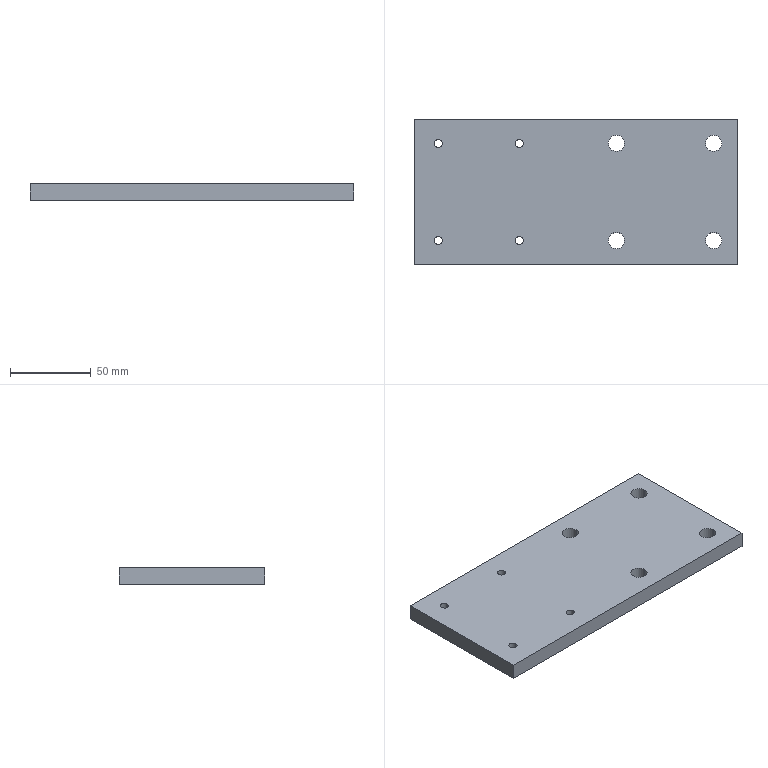Part | SolidWorks | features HoleWzd 2, ICE 2, Extrusion 1 | 1 solid | 22 faces | box 200 x 90 x 10 mm | volume 176073 mm3 | cylinder 16 | plane 6 | commonest cylinder face diameters 5 x8 10 x8
STEP:
#1=CARTESIAN_POINT('',(90.,30.,0.));
#2=VERTEX_POINT('',#1);
#3=CARTESIAN_POINT('',(80.,30.,0.));
#4=VERTEX_POINT('',#3);
#5=CARTESIAN_POINT('',(85.,30.,0.));
#6=DIRECTION('',(0.,0.,-1.));
#7=DIRECTION('',(-1.,0.,0.));
#8=AXIS2_PLACEMENT_3D('',#5,#6,#7);
#9=CIRCLE('',#8,5.);
#10=EDGE_CURVE('',#2,#4,#9,.T.);
#11=ORIENTED_EDGE('',*,*,#10,.T.);
#12=CARTESIAN_POINT('',(80.,30.,10.));
#13=VERTEX_POINT('',#12);
#14=CARTESIAN_POINT('',(80.,30.,10.));
#15=DIRECTION('',(0.,0.,1.));
#16=VECTOR('',#15,1000.);
#17=LINE('',#14,#16);
#18=EDGE_CURVE('',#4,#13,#17,.T.);
#19=ORIENTED_EDGE('',*,*,#18,.T.);
#20=CARTESIAN_POINT('',(90.,30.,10.));
#21=VERTEX_POINT('',#20);
#22=CARTESIAN_POINT('',(85.,30.,10.));
#23=DIRECTION('',(0.,0.,1.));
#24=DIRECTION('',(1.,0.,0.));
#25=AXIS2_PLACEMENT_3D('',#22,#23,#24);
#26=CIRCLE('',#25,5.);
#27=EDGE_CURVE('',#13,#21,#26,.T.);
#28=ORIENTED_EDGE('',*,*,#27,.T.);
#29=CARTESIAN_POINT('',(90.,30.,10.));
#30=DIRECTION('',(0.,0.,1.));
#31=VECTOR('',#30,1000.);
#32=LINE('',#29,#31);
#33=EDGE_CURVE('',#2,#21,#32,.T.);
#34=ORIENTED_EDGE('',*,*,#33,.F.);
#35=EDGE_LOOP('',(#11,#19,#28,#34));
#36=FACE_OUTER_BOUND('',#35,.T.);
#37=CARTESIAN_POINT('',(85.,30.,10.));
#38=DIRECTION('',(0.,0.,1.));
#39=DIRECTION('',(1.,0.,0.));
#40=AXIS2_PLACEMENT_3D('',#37,#38,#39);
#41=CYLINDRICAL_SURFACE('',#40,5.);
#42=ADVANCED_FACE('',(#36),#41,.F.);
#43=CARTESIAN_POINT('',(30.,-30.,0.));
#44=VERTEX_POINT('',#43);
#45=CARTESIAN_POINT('',(20.,-30.,0.));
#46=VERTEX_POINT('',#45);
#47=CARTESIAN_POINT('',(25.,-30.,0.));
#48=DIRECTION('',(0.,0.,-1.));
#49=DIRECTION('',(-1.,0.,0.));
#50=AXIS2_PLACEMENT_3D('',#47,#48,#49);
#51=CIRCLE('',#50,5.);
#52=EDGE_CURVE('',#44,#46,#51,.T.);
#53=ORIENTED_EDGE('',*,*,#52,.T.);
#54=CARTESIAN_POINT('',(20.,-30.,10.));
#55=VERTEX_POINT('',#54);
#56=CARTESIAN_POINT('',(20.,-30.,10.));
#57=DIRECTION('',(0.,0.,1.));
#58=VECTOR('',#57,1000.);
#59=LINE('',#56,#58);
#60=EDGE_CURVE('',#46,#55,#59,.T.);
#61=ORIENTED_EDGE('',*,*,#60,.T.);
#62=CARTESIAN_POINT('',(30.,-30.,10.));
#63=VERTEX_POINT('',#62);
#64=CARTESIAN_POINT('',(25.,-30.,10.));
#65=DIRECTION('',(0.,0.,1.));
#66=DIRECTION('',(1.,0.,0.));
#67=AXIS2_PLACEMENT_3D('',#64,#65,#66);
#68=CIRCLE('',#67,5.);
#69=EDGE_CURVE('',#55,#63,#68,.T.);
#70=ORIENTED_EDGE('',*,*,#69,.T.);
#71=CARTESIAN_POINT('',(30.,-30.,10.));
#72=DIRECTION('',(0.,0.,1.));
#73=VECTOR('',#72,1000.);
#74=LINE('',#71,#73);
#75=EDGE_CURVE('',#44,#63,#74,.T.);
#76=ORIENTED_EDGE('',*,*,#75,.F.);
#77=EDGE_LOOP('',(#53,#61,#70,#76));
#78=FACE_OUTER_BOUND('',#77,.T.);
#79=CARTESIAN_POINT('',(25.,-30.,10.));
#80=DIRECTION('',(0.,0.,1.));
#81=DIRECTION('',(1.,0.,0.));
#82=AXIS2_PLACEMENT_3D('',#79,#80,#81);
#83=CYLINDRICAL_SURFACE('',#82,5.);
#84=ADVANCED_FACE('',(#78),#83,.F.);
#85=CARTESIAN_POINT('',(30.,30.,0.));
#86=VERTEX_POINT('',#85);
#87=CARTESIAN_POINT('',(20.,30.,0.));
#88=VERTEX_POINT('',#87);
#89=CARTESIAN_POINT('',(25.,30.,0.));
#90=DIRECTION('',(0.,0.,-1.));
#91=DIRECTION('',(-1.,0.,0.));
#92=AXIS2_PLACEMENT_3D('',#89,#90,#91);
#93=CIRCLE('',#92,5.);
#94=EDGE_CURVE('',#86,#88,#93,.T.);
#95=ORIENTED_EDGE('',*,*,#94,.T.);
#96=CARTESIAN_POINT('',(20.,30.,10.));
#97=VERTEX_POINT('',#96);
#98=CARTESIAN_POINT('',(20.,30.,10.));
#99=DIRECTION('',(0.,0.,1.));
#100=VECTOR('',#99,1000.);
#101=LINE('',#98,#100);
#102=EDGE_CURVE('',#88,#97,#101,.T.);
#103=ORIENTED_EDGE('',*,*,#102,.T.);
#104=CARTESIAN_POINT('',(30.,30.,10.));
#105=VERTEX_POINT('',#104);
#106=CARTESIAN_POINT('',(25.,30.,10.));
#107=DIRECTION('',(0.,0.,1.));
#108=DIRECTION('',(1.,0.,0.));
#109=AXIS2_PLACEMENT_3D('',#106,#107,#108);
#110=CIRCLE('',#109,5.);
#111=EDGE_CURVE('',#97,#105,#110,.T.);
#112=ORIENTED_EDGE('',*,*,#111,.T.);
#113=CARTESIAN_POINT('',(30.,30.,10.));
#114=DIRECTION('',(0.,0.,1.));
#115=VECTOR('',#114,1000.);
#116=LINE('',#113,#115);
#117=EDGE_CURVE('',#86,#105,#116,.T.);
#118=ORIENTED_EDGE('',*,*,#117,.F.);
#119=EDGE_LOOP('',(#95,#103,#112,#118));
#120=FACE_OUTER_BOUND('',#119,.T.);
#121=CARTESIAN_POINT('',(25.,30.,10.));
#122=DIRECTION('',(0.,0.,1.));
#123=DIRECTION('',(1.,0.,0.));
#124=AXIS2_PLACEMENT_3D('',#121,#122,#123);
#125=CYLINDRICAL_SURFACE('',#124,5.);
#126=ADVANCED_FACE('',(#120),#125,.F.);
#127=CARTESIAN_POINT('',(90.,-30.,0.));
#128=VERTEX_POINT('',#127);
#129=CARTESIAN_POINT('',(80.,-30.,0.));
#130=VERTEX_POINT('',#129);
#131=CARTESIAN_POINT('',(85.,-30.,0.));
#132=DIRECTION('',(0.,0.,-1.));
#133=DIRECTION('',(-1.,0.,0.));
#134=AXIS2_PLACEMENT_3D('',#131,#132,#133);
#135=CIRCLE('',#134,5.);
#136=EDGE_CURVE('',#128,#130,#135,.T.);
#137=ORIENTED_EDGE('',*,*,#136,.T.);
#138=CARTESIAN_POINT('',(80.,-30.,10.));
#139=VERTEX_POINT('',#138);
#140=CARTESIAN_POINT('',(80.,-30.,10.));
#141=DIRECTION('',(0.,0.,1.));
#142=VECTOR('',#141,1000.);
#143=LINE('',#140,#142);
#144=EDGE_CURVE('',#130,#139,#143,.T.);
#145=ORIENTED_EDGE('',*,*,#144,.T.);
#146=CARTESIAN_POINT('',(90.,-30.,10.));
#147=VERTEX_POINT('',#146);
#148=CARTESIAN_POINT('',(85.,-30.,10.));
#149=DIRECTION('',(0.,0.,1.));
#150=DIRECTION('',(1.,0.,0.));
#151=AXIS2_PLACEMENT_3D('',#148,#149,#150);
#152=CIRCLE('',#151,5.);
#153=EDGE_CURVE('',#139,#147,#152,.T.);
#154=ORIENTED_EDGE('',*,*,#153,.T.);
#155=CARTESIAN_POINT('',(90.,-30.,10.));
#156=DIRECTION('',(0.,0.,1.));
#157=VECTOR('',#156,1000.);
#158=LINE('',#155,#157);
#159=EDGE_CURVE('',#128,#147,#158,.T.);
#160=ORIENTED_EDGE('',*,*,#159,.F.);
#161=EDGE_LOOP('',(#137,#145,#154,#160));
#162=FACE_OUTER_BOUND('',#161,.T.);
#163=CARTESIAN_POINT('',(85.,-30.,10.));
#164=DIRECTION('',(0.,0.,1.));
#165=DIRECTION('',(1.,0.,0.));
#166=AXIS2_PLACEMENT_3D('',#163,#164,#165);
#167=CYLINDRICAL_SURFACE('',#166,5.);
#168=ADVANCED_FACE('',(#162),#167,.F.);
#169=CARTESIAN_POINT('',(-32.5,-30.,10.));
#170=VERTEX_POINT('',#169);
#171=CARTESIAN_POINT('',(-37.5,-30.,10.));
#172=VERTEX_POINT('',#171);
#173=CARTESIAN_POINT('',(-35.,-30.,10.));
#174=DIRECTION('',(0.,0.,-1.));
#175=DIRECTION('',(-1.,0.,0.));
#176=AXIS2_PLACEMENT_3D('',#173,#174,#175);
#177=CIRCLE('',#176,2.5);
#178=EDGE_CURVE('',#170,#172,#177,.T.);
#179=ORIENTED_EDGE('',*,*,#178,.F.);
#180=CARTESIAN_POINT('',(-32.5,-30.,0.));
#181=VERTEX_POINT('',#180);
#182=CARTESIAN_POINT('',(-32.5,-30.,0.));
#183=DIRECTION('',(0.,0.,-1.));
#184=VECTOR('',#183,1000.);
#185=LINE('',#182,#184);
#186=EDGE_CURVE('',#170,#181,#185,.T.);
#187=ORIENTED_EDGE('',*,*,#186,.T.);
#188=CARTESIAN_POINT('',(-37.5,-30.,0.));
#189=VERTEX_POINT('',#188);
#190=CARTESIAN_POINT('',(-35.,-30.,0.));
#191=DIRECTION('',(0.,0.,-1.));
#192=DIRECTION('',(-1.,0.,0.));
#193=AXIS2_PLACEMENT_3D('',#190,#191,#192);
#194=CIRCLE('',#193,2.5);
#195=EDGE_CURVE('',#181,#189,#194,.T.);
#196=ORIENTED_EDGE('',*,*,#195,.T.);
#197=CARTESIAN_POINT('',(-37.5,-30.,0.));
#198=DIRECTION('',(0.,0.,-1.));
#199=VECTOR('',#198,1000.);
#200=LINE('',#197,#199);
#201=EDGE_CURVE('',#172,#189,#200,.T.);
#202=ORIENTED_EDGE('',*,*,#201,.F.);
#203=EDGE_LOOP('',(#179,#187,#196,#202));
#204=FACE_OUTER_BOUND('',#203,.T.);
#205=CARTESIAN_POINT('',(-35.,-30.,0.));
#206=DIRECTION('',(0.,0.,-1.));
#207=DIRECTION('',(-1.,0.,0.));
#208=AXIS2_PLACEMENT_3D('',#205,#206,#207);
#209=CYLINDRICAL_SURFACE('',#208,2.5);
#210=ADVANCED_FACE('',(#204),#209,.F.);
#211=CARTESIAN_POINT('',(-82.5,-30.,10.));
#212=VERTEX_POINT('',#211);
#213=CARTESIAN_POINT('',(-87.5,-30.,10.));
#214=VERTEX_POINT('',#213);
#215=CARTESIAN_POINT('',(-85.,-30.,10.));
#216=DIRECTION('',(0.,0.,-1.));
#217=DIRECTION('',(-1.,0.,0.));
#218=AXIS2_PLACEMENT_3D('',#215,#216,#217);
#219=CIRCLE('',#218,2.5);
#220=EDGE_CURVE('',#212,#214,#219,.T.);
#221=ORIENTED_EDGE('',*,*,#220,.F.);
#222=CARTESIAN_POINT('',(-82.5,-30.,0.));
#223=VERTEX_POINT('',#222);
#224=CARTESIAN_POINT('',(-82.5,-30.,0.));
#225=DIRECTION('',(0.,0.,-1.));
#226=VECTOR('',#225,1000.);
#227=LINE('',#224,#226);
#228=EDGE_CURVE('',#212,#223,#227,.T.);
#229=ORIENTED_EDGE('',*,*,#228,.T.);
#230=CARTESIAN_POINT('',(-87.5,-30.,0.));
#231=VERTEX_POINT('',#230);
#232=CARTESIAN_POINT('',(-85.,-30.,0.));
#233=DIRECTION('',(0.,0.,-1.));
#234=DIRECTION('',(-1.,0.,0.));
#235=AXIS2_PLACEMENT_3D('',#232,#233,#234);
#236=CIRCLE('',#235,2.5);
#237=EDGE_CURVE('',#223,#231,#236,.T.);
#238=ORIENTED_EDGE('',*,*,#237,.T.);
#239=CARTESIAN_POINT('',(-87.5,-30.,0.));
#240=DIRECTION('',(0.,0.,-1.));
#241=VECTOR('',#240,1000.);
#242=LINE('',#239,#241);
#243=EDGE_CURVE('',#214,#231,#242,.T.);
#244=ORIENTED_EDGE('',*,*,#243,.F.);
#245=EDGE_LOOP('',(#221,#229,#238,#244));
#246=FACE_OUTER_BOUND('',#245,.T.);
#247=CARTESIAN_POINT('',(-85.,-30.,0.));
#248=DIRECTION('',(0.,0.,-1.));
#249=DIRECTION('',(-1.,0.,0.));
#250=AXIS2_PLACEMENT_3D('',#247,#248,#249);
#251=CYLINDRICAL_SURFACE('',#250,2.5);
#252=ADVANCED_FACE('',(#246),#251,.F.);
#253=CARTESIAN_POINT('',(-32.5,30.,10.));
#254=VERTEX_POINT('',#253);
#255=CARTESIAN_POINT('',(-37.5,30.,10.));
#256=VERTEX_POINT('',#255);
#257=CARTESIAN_POINT('',(-35.,30.,10.));
#258=DIRECTION('',(0.,0.,-1.));
#259=DIRECTION('',(-1.,0.,0.));
#260=AXIS2_PLACEMENT_3D('',#257,#258,#259);
#261=CIRCLE('',#260,2.5);
#262=EDGE_CURVE('',#254,#256,#261,.T.);
#263=ORIENTED_EDGE('',*,*,#262,.F.);
#264=CARTESIAN_POINT('',(-32.5,30.,0.));
#265=VERTEX_POINT('',#264);
#266=CARTESIAN_POINT('',(-32.5,30.,0.));
#267=DIRECTION('',(0.,0.,-1.));
#268=VECTOR('',#267,1000.);
#269=LINE('',#266,#268);
#270=EDGE_CURVE('',#254,#265,#269,.T.);
#271=ORIENTED_EDGE('',*,*,#270,.T.);
#272=CARTESIAN_POINT('',(-37.5,30.,0.));
#273=VERTEX_POINT('',#272);
#274=CARTESIAN_POINT('',(-35.,30.,0.));
#275=DIRECTION('',(0.,0.,-1.));
#276=DIRECTION('',(-1.,0.,0.));
#277=AXIS2_PLACEMENT_3D('',#274,#275,#276);
#278=CIRCLE('',#277,2.5);
#279=EDGE_CURVE('',#265,#273,#278,.T.);
#280=ORIENTED_EDGE('',*,*,#279,.T.);
#281=CARTESIAN_POINT('',(-37.5,30.,0.));
#282=DIRECTION('',(0.,0.,-1.));
#283=VECTOR('',#282,1000.);
#284=LINE('',#281,#283);
#285=EDGE_CURVE('',#256,#273,#284,.T.);
#286=ORIENTED_EDGE('',*,*,#285,.F.);
#287=EDGE_LOOP('',(#263,#271,#280,#286));
#288=FACE_OUTER_BOUND('',#287,.T.);
#289=CARTESIAN_POINT('',(-35.,30.,0.));
#290=DIRECTION('',(0.,0.,-1.));
#291=DIRECTION('',(-1.,0.,0.));
#292=AXIS2_PLACEMENT_3D('',#289,#290,#291);
#293=CYLINDRICAL_SURFACE('',#292,2.5);
#294=ADVANCED_FACE('',(#288),#293,.F.);
#295=CARTESIAN_POINT('',(-82.5,30.,10.));
#296=VERTEX_POINT('',#295);
#297=CARTESIAN_POINT('',(-87.5,30.,10.));
#298=VERTEX_POINT('',#297);
#299=CARTESIAN_POINT('',(-85.,30.,10.));
#300=DIRECTION('',(0.,0.,-1.));
#301=DIRECTION('',(-1.,0.,0.));
#302=AXIS2_PLACEMENT_3D('',#299,#300,#301);
#303=CIRCLE('',#302,2.5);
#304=EDGE_CURVE('',#296,#298,#303,.T.);
#305=ORIENTED_EDGE('',*,*,#304,.F.);
#306=CARTESIAN_POINT('',(-82.5,30.,0.));
#307=VERTEX_POINT('',#306);
#308=CARTESIAN_POINT('',(-82.5,30.,0.));
#309=DIRECTION('',(0.,0.,-1.));
#310=VECTOR('',#309,1000.);
#311=LINE('',#308,#310);
#312=EDGE_CURVE('',#296,#307,#311,.T.);
#313=ORIENTED_EDGE('',*,*,#312,.T.);
#314=CARTESIAN_POINT('',(-87.5,30.,0.));
#315=VERTEX_POINT('',#314);
#316=CARTESIAN_POINT('',(-85.,30.,0.));
#317=DIRECTION('',(0.,0.,-1.));
#318=DIRECTION('',(-1.,0.,0.));
#319=AXIS2_PLACEMENT_3D('',#316,#317,#318);
#320=CIRCLE('',#319,2.5);
#321=EDGE_CURVE('',#307,#315,#320,.T.);
#322=ORIENTED_EDGE('',*,*,#321,.T.);
#323=CARTESIAN_POINT('',(-87.5,30.,0.));
#324=DIRECTION('',(0.,0.,-1.));
#325=VECTOR('',#324,1000.);
#326=LINE('',#323,#325);
#327=EDGE_CURVE('',#298,#315,#326,.T.);
#328=ORIENTED_EDGE('',*,*,#327,.F.);
#329=EDGE_LOOP('',(#305,#313,#322,#328));
#330=FACE_OUTER_BOUND('',#329,.T.);
#331=CARTESIAN_POINT('',(-85.,30.,0.));
#332=DIRECTION('',(0.,0.,-1.));
#333=DIRECTION('',(-1.,0.,0.));
#334=AXIS2_PLACEMENT_3D('',#331,#332,#333);
#335=CYLINDRICAL_SURFACE('',#334,2.5);
#336=ADVANCED_FACE('',(#330),#335,.F.);
#337=CARTESIAN_POINT('',(100.,-45.,0.));
#338=VERTEX_POINT('',#337);
#339=CARTESIAN_POINT('',(100.,45.,0.));
#340=VERTEX_POINT('',#339);
#341=CARTESIAN_POINT('',(100.,-45.,0.));
#342=DIRECTION('',(0.,1.,0.));
#343=VECTOR('',#342,1000.);
#344=LINE('',#341,#343);
#345=EDGE_CURVE('',#338,#340,#344,.T.);
#346=ORIENTED_EDGE('',*,*,#345,.T.);
#347=CARTESIAN_POINT('',(100.,45.,10.));
#348=VERTEX_POINT('',#347);
#349=CARTESIAN_POINT('',(100.,45.,10.));
#350=DIRECTION('',(0.,0.,-1.));
#351=VECTOR('',#350,1000.);
#352=LINE('',#349,#351);
#353=EDGE_CURVE('',#348,#340,#352,.T.);
#354=ORIENTED_EDGE('',*,*,#353,.F.);
#355=CARTESIAN_POINT('',(100.,-45.,10.));
#356=VERTEX_POINT('',#355);
#357=CARTESIAN_POINT('',(100.,-45.,10.));
#358=DIRECTION('',(0.,1.,0.));
#359=VECTOR('',#358,1000.);
#360=LINE('',#357,#359);
#361=EDGE_CURVE('',#356,#348,#360,.T.);
#362=ORIENTED_EDGE('',*,*,#361,.F.);
#363=CARTESIAN_POINT('',(100.,-45.,10.));
#364=DIRECTION('',(0.,0.,-1.));
#365=VECTOR('',#364,1000.);
#366=LINE('',#363,#365);
#367=EDGE_CURVE('',#356,#338,#366,.T.);
#368=ORIENTED_EDGE('',*,*,#367,.T.);
#369=EDGE_LOOP('',(#346,#354,#362,#368));
#370=FACE_OUTER_BOUND('',#369,.T.);
#371=CARTESIAN_POINT('',(100.,-45.,10.));
#372=DIRECTION('',(-1.,0.,0.));
#373=DIRECTION('',(0.,0.,1.));
#374=AXIS2_PLACEMENT_3D('',#371,#372,#373);
#375=PLANE('',#374);
#376=ADVANCED_FACE('',(#370),#375,.F.);
#377=CARTESIAN_POINT('',(-100.,45.,0.));
#378=VERTEX_POINT('',#377);
#379=CARTESIAN_POINT('',(-100.,45.,0.));
#380=DIRECTION('',(-1.,0.,0.));
#381=VECTOR('',#380,1000.);
#382=LINE('',#379,#381);
#383=EDGE_CURVE('',#340,#378,#382,.T.);
#384=ORIENTED_EDGE('',*,*,#383,.T.);
#385=CARTESIAN_POINT('',(-100.,45.,10.));
#386=VERTEX_POINT('',#385);
#387=CARTESIAN_POINT('',(-100.,45.,10.));
#388=DIRECTION('',(0.,0.,-1.));
#389=VECTOR('',#388,1000.);
#390=LINE('',#387,#389);
#391=EDGE_CURVE('',#386,#378,#390,.T.);
#392=ORIENTED_EDGE('',*,*,#391,.F.);
#393=CARTESIAN_POINT('',(-100.,45.,10.));
#394=DIRECTION('',(-1.,0.,0.));
#395=VECTOR('',#394,1000.);
#396=LINE('',#393,#395);
#397=EDGE_CURVE('',#348,#386,#396,.T.);
#398=ORIENTED_EDGE('',*,*,#397,.F.);
#399=ORIENTED_EDGE('',*,*,#353,.T.);
#400=EDGE_LOOP('',(#384,#392,#398,#399));
#401=FACE_OUTER_BOUND('',#400,.T.);
#402=CARTESIAN_POINT('',(-100.,45.,10.));
#403=DIRECTION('',(0.,-1.,0.));
#404=DIRECTION('',(0.,0.,-1.));
#405=AXIS2_PLACEMENT_3D('',#402,#403,#404);
#406=PLANE('',#405);
#407=ADVANCED_FACE('',(#401),#406,.F.);
#408=CARTESIAN_POINT('',(-100.,-45.,0.));
#409=VERTEX_POINT('',#408);
#410=CARTESIAN_POINT('',(-100.,-45.,0.));
#411=DIRECTION('',(0.,-1.,0.));
#412=VECTOR('',#411,1000.);
#413=LINE('',#410,#412);
#414=EDGE_CURVE('',#378,#409,#413,.T.);
#415=ORIENTED_EDGE('',*,*,#414,.T.);
#416=CARTESIAN_POINT('',(-100.,-45.,10.));
#417=VERTEX_POINT('',#416);
#418=CARTESIAN_POINT('',(-100.,-45.,10.));
#419=DIRECTION('',(0.,0.,-1.));
#420=VECTOR('',#419,1000.);
#421=LINE('',#418,#420);
#422=EDGE_CURVE('',#417,#409,#421,.T.);
#423=ORIENTED_EDGE('',*,*,#422,.F.);
#424=CARTESIAN_POINT('',(-100.,-45.,10.));
#425=DIRECTION('',(0.,-1.,0.));
#426=VECTOR('',#425,1000.);
#427=LINE('',#424,#426);
#428=EDGE_CURVE('',#386,#417,#427,.T.);
#429=ORIENTED_EDGE('',*,*,#428,.F.);
#430=ORIENTED_EDGE('',*,*,#391,.T.);
#431=EDGE_LOOP('',(#415,#423,#429,#430));
#432=FACE_OUTER_BOUND('',#431,.T.);
#433=CARTESIAN_POINT('',(-100.,-45.,10.));
#434=DIRECTION('',(1.,0.,0.));
#435=DIRECTION('',(0.,0.,-1.));
#436=AXIS2_PLACEMENT_3D('',#433,#434,#435);
#437=PLANE('',#436);
#438=ADVANCED_FACE('',(#432),#437,.F.);
#439=CARTESIAN_POINT('',(-100.,-45.,0.));
#440=DIRECTION('',(1.,0.,0.));
#441=VECTOR('',#440,1000.);
#442=LINE('',#439,#441);
#443=EDGE_CURVE('',#409,#338,#442,.T.);
#444=ORIENTED_EDGE('',*,*,#443,.T.);
#445=ORIENTED_EDGE('',*,*,#367,.F.);
#446=CARTESIAN_POINT('',(-100.,-45.,10.));
#447=DIRECTION('',(1.,0.,0.));
#448=VECTOR('',#447,1000.);
#449=LINE('',#446,#448);
#450=EDGE_CURVE('',#417,#356,#449,.T.);
#451=ORIENTED_EDGE('',*,*,#450,.F.);
#452=ORIENTED_EDGE('',*,*,#422,.T.);
#453=EDGE_LOOP('',(#444,#445,#451,#452));
#454=FACE_OUTER_BOUND('',#453,.T.);
#455=CARTESIAN_POINT('',(-100.,-45.,10.));
#456=DIRECTION('',(0.,1.,0.));
#457=DIRECTION('',(0.,0.,1.));
#458=AXIS2_PLACEMENT_3D('',#455,#456,#457);
#459=PLANE('',#458);
#460=ADVANCED_FACE('',(#454),#459,.F.);
#461=CARTESIAN_POINT('',(85.,30.,10.));
#462=DIRECTION('',(0.,0.,1.));
#463=DIRECTION('',(1.,0.,0.));
#464=AXIS2_PLACEMENT_3D('',#461,#462,#463);
#465=CIRCLE('',#464,5.);
#466=EDGE_CURVE('',#21,#13,#465,.T.);
#467=ORIENTED_EDGE('',*,*,#466,.F.);
#468=ORIENTED_EDGE('',*,*,#27,.F.);
#469=EDGE_LOOP('',(#467,#468));
#470=FACE_BOUND('',#469,.T.);
#471=CARTESIAN_POINT('',(25.,-30.,10.));
#472=DIRECTION('',(0.,0.,1.));
#473=DIRECTION('',(1.,0.,0.));
#474=AXIS2_PLACEMENT_3D('',#471,#472,#473);
#475=CIRCLE('',#474,5.);
#476=EDGE_CURVE('',#63,#55,#475,.T.);
#477=ORIENTED_EDGE('',*,*,#476,.F.);
#478=ORIENTED_EDGE('',*,*,#69,.F.);
#479=EDGE_LOOP('',(#477,#478));
#480=FACE_BOUND('',#479,.T.);
#481=CARTESIAN_POINT('',(25.,30.,10.));
#482=DIRECTION('',(0.,0.,1.));
#483=DIRECTION('',(1.,0.,0.));
#484=AXIS2_PLACEMENT_3D('',#481,#482,#483);
#485=CIRCLE('',#484,5.);
#486=EDGE_CURVE('',#105,#97,#485,.T.);
#487=ORIENTED_EDGE('',*,*,#486,.F.);
#488=ORIENTED_EDGE('',*,*,#111,.F.);
#489=EDGE_LOOP('',(#487,#488));
#490=FACE_BOUND('',#489,.T.);
#491=CARTESIAN_POINT('',(85.,-30.,10.));
#492=DIRECTION('',(0.,0.,1.));
#493=DIRECTION('',(1.,0.,0.));
#494=AXIS2_PLACEMENT_3D('',#491,#492,#493);
#495=CIRCLE('',#494,5.);
#496=EDGE_CURVE('',#147,#139,#495,.T.);
#497=ORIENTED_EDGE('',*,*,#496,.F.);
#498=ORIENTED_EDGE('',*,*,#153,.F.);
#499=EDGE_LOOP('',(#497,#498));
#500=FACE_BOUND('',#499,.T.);
#501=CARTESIAN_POINT('',(-35.,-30.,10.));
#502=DIRECTION('',(0.,0.,-1.));
#503=DIRECTION('',(-1.,0.,0.));
#504=AXIS2_PLACEMENT_3D('',#501,#502,#503);
#505=CIRCLE('',#504,2.5);
#506=EDGE_CURVE('',#172,#170,#505,.T.);
#507=ORIENTED_EDGE('',*,*,#506,.T.);
#508=ORIENTED_EDGE('',*,*,#178,.T.);
#509=EDGE_LOOP('',(#507,#508));
#510=FACE_BOUND('',#509,.T.);
#511=CARTESIAN_POINT('',(-85.,-30.,10.));
#512=DIRECTION('',(0.,0.,-1.));
#513=DIRECTION('',(-1.,0.,0.));
#514=AXIS2_PLACEMENT_3D('',#511,#512,#513);
#515=CIRCLE('',#514,2.5);
#516=EDGE_CURVE('',#214,#212,#515,.T.);
#517=ORIENTED_EDGE('',*,*,#516,.T.);
#518=ORIENTED_EDGE('',*,*,#220,.T.);
#519=EDGE_LOOP('',(#517,#518));
#520=FACE_BOUND('',#519,.T.);
#521=CARTESIAN_POINT('',(-35.,30.,10.));
#522=DIRECTION('',(0.,0.,-1.));
#523=DIRECTION('',(-1.,0.,0.));
#524=AXIS2_PLACEMENT_3D('',#521,#522,#523);
#525=CIRCLE('',#524,2.5);
#526=EDGE_CURVE('',#256,#254,#525,.T.);
#527=ORIENTED_EDGE('',*,*,#526,.T.);
#528=ORIENTED_EDGE('',*,*,#262,.T.);
#529=EDGE_LOOP('',(#527,#528));
#530=FACE_BOUND('',#529,.T.);
#531=CARTESIAN_POINT('',(-85.,30.,10.));
#532=DIRECTION('',(0.,0.,-1.));
#533=DIRECTION('',(-1.,0.,0.));
#534=AXIS2_PLACEMENT_3D('',#531,#532,#533);
#535=CIRCLE('',#534,2.5);
#536=EDGE_CURVE('',#298,#296,#535,.T.);
#537=ORIENTED_EDGE('',*,*,#536,.T.);
#538=ORIENTED_EDGE('',*,*,#304,.T.);
#539=EDGE_LOOP('',(#537,#538));
#540=FACE_BOUND('',#539,.T.);
#541=ORIENTED_EDGE('',*,*,#361,.T.);
#542=ORIENTED_EDGE('',*,*,#397,.T.);
#543=ORIENTED_EDGE('',*,*,#428,.T.);
#544=ORIENTED_EDGE('',*,*,#450,.T.);
#545=EDGE_LOOP('',(#541,#542,#543,#544));
#546=FACE_OUTER_BOUND('',#545,.T.);
#547=CARTESIAN_POINT('',(0.,0.,10.));
#548=DIRECTION('',(0.,0.,-1.));
#549=DIRECTION('',(-1.,0.,0.));
#550=AXIS2_PLACEMENT_3D('',#547,#548,#549);
#551=PLANE('',#550);
#552=ADVANCED_FACE('',(#470,#480,#490,#500,#510,#520,#530,#540,#546),#551,.F.);
#553=ORIENTED_EDGE('',*,*,#10,.F.);
#554=CARTESIAN_POINT('',(85.,30.,0.));
#555=DIRECTION('',(0.,0.,-1.));
#556=DIRECTION('',(-1.,0.,0.));
#557=AXIS2_PLACEMENT_3D('',#554,#555,#556);
#558=CIRCLE('',#557,5.);
#559=EDGE_CURVE('',#4,#2,#558,.T.);
#560=ORIENTED_EDGE('',*,*,#559,.F.);
#561=EDGE_LOOP('',(#553,#560));
#562=FACE_BOUND('',#561,.T.);
#563=ORIENTED_EDGE('',*,*,#52,.F.);
#564=CARTESIAN_POINT('',(25.,-30.,0.));
#565=DIRECTION('',(0.,0.,-1.));
#566=DIRECTION('',(-1.,0.,0.));
#567=AXIS2_PLACEMENT_3D('',#564,#565,#566);
#568=CIRCLE('',#567,5.);
#569=EDGE_CURVE('',#46,#44,#568,.T.);
#570=ORIENTED_EDGE('',*,*,#569,.F.);
#571=EDGE_LOOP('',(#563,#570));
#572=FACE_BOUND('',#571,.T.);
#573=ORIENTED_EDGE('',*,*,#94,.F.);
#574=CARTESIAN_POINT('',(25.,30.,0.));
#575=DIRECTION('',(0.,0.,-1.));
#576=DIRECTION('',(-1.,0.,0.));
#577=AXIS2_PLACEMENT_3D('',#574,#575,#576);
#578=CIRCLE('',#577,5.);
#579=EDGE_CURVE('',#88,#86,#578,.T.);
#580=ORIENTED_EDGE('',*,*,#579,.F.);
#581=EDGE_LOOP('',(#573,#580));
#582=FACE_BOUND('',#581,.T.);
#583=ORIENTED_EDGE('',*,*,#136,.F.);
#584=CARTESIAN_POINT('',(85.,-30.,0.));
#585=DIRECTION('',(0.,0.,-1.));
#586=DIRECTION('',(-1.,0.,0.));
#587=AXIS2_PLACEMENT_3D('',#584,#585,#586);
#588=CIRCLE('',#587,5.);
#589=EDGE_CURVE('',#130,#128,#588,.T.);
#590=ORIENTED_EDGE('',*,*,#589,.F.);
#591=EDGE_LOOP('',(#583,#590));
#592=FACE_BOUND('',#591,.T.);
#593=CARTESIAN_POINT('',(-35.,-30.,0.));
#594=DIRECTION('',(0.,0.,-1.));
#595=DIRECTION('',(-1.,0.,0.));
#596=AXIS2_PLACEMENT_3D('',#593,#594,#595);
#597=CIRCLE('',#596,2.5);
#598=EDGE_CURVE('',#189,#181,#597,.T.);
#599=ORIENTED_EDGE('',*,*,#598,.F.);
#600=ORIENTED_EDGE('',*,*,#195,.F.);
#601=EDGE_LOOP('',(#599,#600));
#602=FACE_BOUND('',#601,.T.);
#603=CARTESIAN_POINT('',(-85.,-30.,0.));
#604=DIRECTION('',(0.,0.,-1.));
#605=DIRECTION('',(-1.,0.,0.));
#606=AXIS2_PLACEMENT_3D('',#603,#604,#605);
#607=CIRCLE('',#606,2.5);
#608=EDGE_CURVE('',#231,#223,#607,.T.);
#609=ORIENTED_EDGE('',*,*,#608,.F.);
#610=ORIENTED_EDGE('',*,*,#237,.F.);
#611=EDGE_LOOP('',(#609,#610));
#612=FACE_BOUND('',#611,.T.);
#613=CARTESIAN_POINT('',(-35.,30.,0.));
#614=DIRECTION('',(0.,0.,-1.));
#615=DIRECTION('',(-1.,0.,0.));
#616=AXIS2_PLACEMENT_3D('',#613,#614,#615);
#617=CIRCLE('',#616,2.5);
#618=EDGE_CURVE('',#273,#265,#617,.T.);
#619=ORIENTED_EDGE('',*,*,#618,.F.);
#620=ORIENTED_EDGE('',*,*,#279,.F.);
#621=EDGE_LOOP('',(#619,#620));
#622=FACE_BOUND('',#621,.T.);
#623=CARTESIAN_POINT('',(-85.,30.,0.));
#624=DIRECTION('',(0.,0.,-1.));
#625=DIRECTION('',(-1.,0.,0.));
#626=AXIS2_PLACEMENT_3D('',#623,#624,#625);
#627=CIRCLE('',#626,2.5);
#628=EDGE_CURVE('',#315,#307,#627,.T.);
#629=ORIENTED_EDGE('',*,*,#628,.F.);
#630=ORIENTED_EDGE('',*,*,#321,.F.);
#631=EDGE_LOOP('',(#629,#630));
#632=FACE_BOUND('',#631,.T.);
#633=ORIENTED_EDGE('',*,*,#345,.F.);
#634=ORIENTED_EDGE('',*,*,#443,.F.);
#635=ORIENTED_EDGE('',*,*,#414,.F.);
#636=ORIENTED_EDGE('',*,*,#383,.F.);
#637=EDGE_LOOP('',(#633,#634,#635,#636));
#638=FACE_OUTER_BOUND('',#637,.T.);
#639=CARTESIAN_POINT('',(0.,0.,0.));
#640=DIRECTION('',(0.,0.,-1.));
#641=DIRECTION('',(-1.,0.,0.));
#642=AXIS2_PLACEMENT_3D('',#639,#640,#641);
#643=PLANE('',#642);
#644=ADVANCED_FACE('',(#562,#572,#582,#592,#602,#612,#622,#632,#638),#643,.T.);
#645=ORIENTED_EDGE('',*,*,#312,.F.);
#646=ORIENTED_EDGE('',*,*,#536,.F.);
#647=ORIENTED_EDGE('',*,*,#327,.T.);
#648=ORIENTED_EDGE('',*,*,#628,.T.);
#649=EDGE_LOOP('',(#645,#646,#647,#648));
#650=FACE_OUTER_BOUND('',#649,.T.);
#651=CARTESIAN_POINT('',(-85.,30.,0.));
#652=DIRECTION('',(0.,0.,-1.));
#653=DIRECTION('',(-1.,0.,0.));
#654=AXIS2_PLACEMENT_3D('',#651,#652,#653);
#655=CYLINDRICAL_SURFACE('',#654,2.5);
#656=ADVANCED_FACE('',(#650),#655,.F.);
#657=ORIENTED_EDGE('',*,*,#270,.F.);
#658=ORIENTED_EDGE('',*,*,#526,.F.);
#659=ORIENTED_EDGE('',*,*,#285,.T.);
#660=ORIENTED_EDGE('',*,*,#618,.T.);
#661=EDGE_LOOP('',(#657,#658,#659,#660));
#662=FACE_OUTER_BOUND('',#661,.T.);
#663=CARTESIAN_POINT('',(-35.,30.,0.));
#664=DIRECTION('',(0.,0.,-1.));
#665=DIRECTION('',(-1.,0.,0.));
#666=AXIS2_PLACEMENT_3D('',#663,#664,#665);
#667=CYLINDRICAL_SURFACE('',#666,2.5);
#668=ADVANCED_FACE('',(#662),#667,.F.);
#669=ORIENTED_EDGE('',*,*,#228,.F.);
#670=ORIENTED_EDGE('',*,*,#516,.F.);
#671=ORIENTED_EDGE('',*,*,#243,.T.);
#672=ORIENTED_EDGE('',*,*,#608,.T.);
#673=EDGE_LOOP('',(#669,#670,#671,#672));
#674=FACE_OUTER_BOUND('',#673,.T.);
#675=CARTESIAN_POINT('',(-85.,-30.,0.));
#676=DIRECTION('',(0.,0.,-1.));
#677=DIRECTION('',(-1.,0.,0.));
#678=AXIS2_PLACEMENT_3D('',#675,#676,#677);
#679=CYLINDRICAL_SURFACE('',#678,2.5);
#680=ADVANCED_FACE('',(#674),#679,.F.);
#681=ORIENTED_EDGE('',*,*,#186,.F.);
#682=ORIENTED_EDGE('',*,*,#506,.F.);
#683=ORIENTED_EDGE('',*,*,#201,.T.);
#684=ORIENTED_EDGE('',*,*,#598,.T.);
#685=EDGE_LOOP('',(#681,#682,#683,#684));
#686=FACE_OUTER_BOUND('',#685,.T.);
#687=CARTESIAN_POINT('',(-35.,-30.,0.));
#688=DIRECTION('',(0.,0.,-1.));
#689=DIRECTION('',(-1.,0.,0.));
#690=AXIS2_PLACEMENT_3D('',#687,#688,#689);
#691=CYLINDRICAL_SURFACE('',#690,2.5);
#692=ADVANCED_FACE('',(#686),#691,.F.);
#693=ORIENTED_EDGE('',*,*,#144,.F.);
#694=ORIENTED_EDGE('',*,*,#589,.T.);
#695=ORIENTED_EDGE('',*,*,#159,.T.);
#696=ORIENTED_EDGE('',*,*,#496,.T.);
#697=EDGE_LOOP('',(#693,#694,#695,#696));
#698=FACE_OUTER_BOUND('',#697,.T.);
#699=CARTESIAN_POINT('',(85.,-30.,10.));
#700=DIRECTION('',(0.,0.,1.));
#701=DIRECTION('',(1.,0.,0.));
#702=AXIS2_PLACEMENT_3D('',#699,#700,#701);
#703=CYLINDRICAL_SURFACE('',#702,5.);
#704=ADVANCED_FACE('',(#698),#703,.F.);
#705=ORIENTED_EDGE('',*,*,#102,.F.);
#706=ORIENTED_EDGE('',*,*,#579,.T.);
#707=ORIENTED_EDGE('',*,*,#117,.T.);
#708=ORIENTED_EDGE('',*,*,#486,.T.);
#709=EDGE_LOOP('',(#705,#706,#707,#708));
#710=FACE_OUTER_BOUND('',#709,.T.);
#711=CARTESIAN_POINT('',(25.,30.,10.));
#712=DIRECTION('',(0.,0.,1.));
#713=DIRECTION('',(1.,0.,0.));
#714=AXIS2_PLACEMENT_3D('',#711,#712,#713);
#715=CYLINDRICAL_SURFACE('',#714,5.);
#716=ADVANCED_FACE('',(#710),#715,.F.);
#717=ORIENTED_EDGE('',*,*,#60,.F.);
#718=ORIENTED_EDGE('',*,*,#569,.T.);
#719=ORIENTED_EDGE('',*,*,#75,.T.);
#720=ORIENTED_EDGE('',*,*,#476,.T.);
#721=EDGE_LOOP('',(#717,#718,#719,#720));
#722=FACE_OUTER_BOUND('',#721,.T.);
#723=CARTESIAN_POINT('',(25.,-30.,10.));
#724=DIRECTION('',(0.,0.,1.));
#725=DIRECTION('',(1.,0.,0.));
#726=AXIS2_PLACEMENT_3D('',#723,#724,#725);
#727=CYLINDRICAL_SURFACE('',#726,5.);
#728=ADVANCED_FACE('',(#722),#727,.F.);
#729=ORIENTED_EDGE('',*,*,#18,.F.);
#730=ORIENTED_EDGE('',*,*,#559,.T.);
#731=ORIENTED_EDGE('',*,*,#33,.T.);
#732=ORIENTED_EDGE('',*,*,#466,.T.);
#733=EDGE_LOOP('',(#729,#730,#731,#732));
#734=FACE_OUTER_BOUND('',#733,.T.);
#735=CARTESIAN_POINT('',(85.,30.,10.));
#736=DIRECTION('',(0.,0.,1.));
#737=DIRECTION('',(1.,0.,0.));
#738=AXIS2_PLACEMENT_3D('',#735,#736,#737);
#739=CYLINDRICAL_SURFACE('',#738,5.);
#740=ADVANCED_FACE('',(#734),#739,.F.);
#741=CLOSED_SHELL('',(#42,#84,#126,#168,#210,#252,#294,#336,#376,#407,#438,#460,#552,#644,#656,#668,#680,#692,#704,#716,#728,#740));
#742=MANIFOLD_SOLID_BREP('',#741);
#743=CARTESIAN_POINT('',(0.,0.,0.));
#744=DIRECTION('',(0.,0.,1.));
#745=DIRECTION('',(1.,0.,0.));
#746=AXIS2_PLACEMENT_3D('',#743,#744,#745);
#747=(LENGTH_UNIT()NAMED_UNIT(*)SI_UNIT(.MILLI.,.METRE.));
#748=UNCERTAINTY_MEASURE_WITH_UNIT(LENGTH_MEASURE(0.00001),#747,'','');
#749=(NAMED_UNIT(*)PLANE_ANGLE_UNIT()SI_UNIT($,.RADIAN.));
#750=(NAMED_UNIT(*)SI_UNIT($,.STERADIAN.)SOLID_ANGLE_UNIT());
#751=(GEOMETRIC_REPRESENTATION_CONTEXT(3)GLOBAL_UNCERTAINTY_ASSIGNED_CONTEXT((#748))GLOBAL_UNIT_ASSIGNED_CONTEXT((#747,#749,#750))REPRESENTATION_CONTEXT('',''));
#752=ADVANCED_BREP_SHAPE_REPRESENTATION('',(#742,#746),#751);